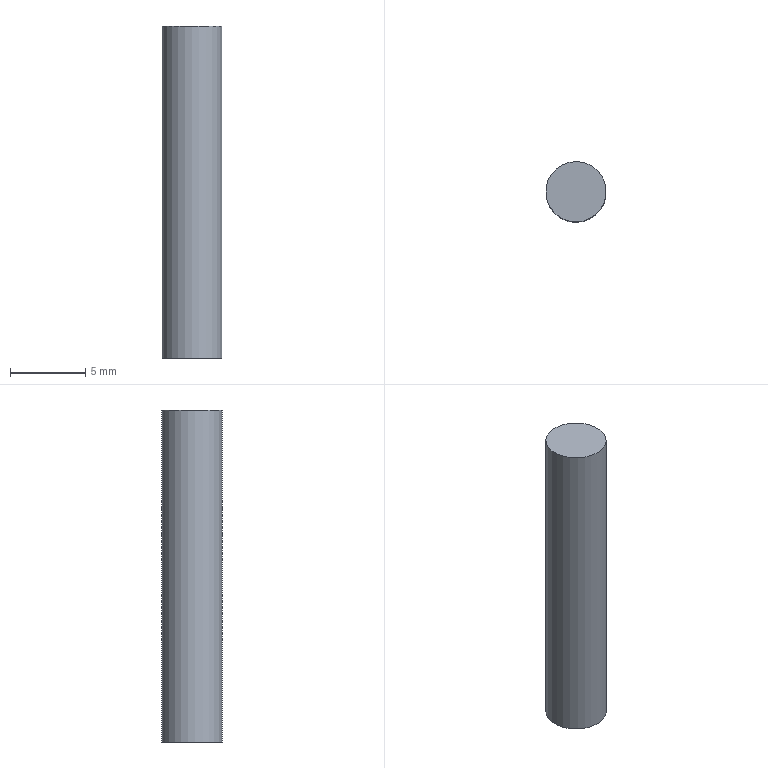Part | NX | features solid 2 | 1 solid | 3 faces | box 4 x 4 x 22 mm | volume 276.46 mm3 | plane 2 | cylinder 1 | commonest cylinder face diameters 4 x1
STEP:
#1=CARTESIAN_POINT('',(-819.874,-95.045,29.));
#2=VERTEX_POINT('',#1);
#3=CARTESIAN_POINT('',(-818.236,-96.192,29.));
#4=DIRECTION('',(0.,0.,1.));
#5=DIRECTION('',(-0.8192,0.5736,0.));
#6=AXIS2_PLACEMENT_3D('',#3,#4,#5);
#7=CIRCLE('',#6,2.);
#8=EDGE_CURVE('',#2,#2,#7,.T.);
#9=ORIENTED_EDGE('',*,*,#8,.F.);
#10=EDGE_LOOP('',(#9));
#11=FACE_BOUND('',#10,.T.);
#12=CARTESIAN_POINT('',(-818.236,-96.192,29.));
#13=DIRECTION('',(0.,0.,-1.));
#14=DIRECTION('',(0.8192,-0.5736,0.));
#15=AXIS2_PLACEMENT_3D('',#12,#13,#14);
#16=PLANE('',#15);
#17=ADVANCED_FACE('',(#11),#16,.T.);
#18=CARTESIAN_POINT('',(-816.597,-97.339,51.));
#19=VERTEX_POINT('',#18);
#20=CARTESIAN_POINT('',(-818.236,-96.192,51.));
#21=DIRECTION('',(0.,0.,-1.));
#22=DIRECTION('',(0.8192,-0.5736,0.));
#23=AXIS2_PLACEMENT_3D('',#20,#21,#22);
#24=CIRCLE('',#23,2.);
#25=EDGE_CURVE('',#19,#19,#24,.T.);
#26=ORIENTED_EDGE('',*,*,#25,.F.);
#27=EDGE_LOOP('',(#26));
#28=FACE_BOUND('',#27,.T.);
#29=CARTESIAN_POINT('',(-818.236,-96.192,51.));
#30=DIRECTION('',(0.,0.,1.));
#31=DIRECTION('',(-0.8192,0.5736,0.));
#32=AXIS2_PLACEMENT_3D('',#29,#30,#31);
#33=PLANE('',#32);
#34=ADVANCED_FACE('',(#28),#33,.T.);
#35=ORIENTED_EDGE('',*,*,#8,.T.);
#36=EDGE_LOOP('',(#35));
#37=FACE_BOUND('',#36,.T.);
#38=ORIENTED_EDGE('',*,*,#25,.T.);
#39=EDGE_LOOP('',(#38));
#40=FACE_BOUND('',#39,.T.);
#41=CARTESIAN_POINT('',(-818.236,-96.192,51.));
#42=DIRECTION('',(0.,0.,-1.));
#43=DIRECTION('',(0.8192,-0.5736,0.));
#44=AXIS2_PLACEMENT_3D('',#41,#42,#43);
#45=CYLINDRICAL_SURFACE('',#44,2.);
#46=ADVANCED_FACE('',(#37,#40),#45,.T.);
#47=CLOSED_SHELL('',(#17,#34,#46));
#48=MANIFOLD_SOLID_BREP('',#47);
#49=(LENGTH_UNIT()NAMED_UNIT(*)SI_UNIT(.MILLI.,.METRE.));
#50=UNCERTAINTY_MEASURE_WITH_UNIT(LENGTH_MEASURE(0.00001),#49,'','');
#51=(NAMED_UNIT(*)PLANE_ANGLE_UNIT()SI_UNIT($,.RADIAN.));
#52=(NAMED_UNIT(*)SI_UNIT($,.STERADIAN.)SOLID_ANGLE_UNIT());
#53=(GEOMETRIC_REPRESENTATION_CONTEXT(3)GLOBAL_UNCERTAINTY_ASSIGNED_CONTEXT((#50))GLOBAL_UNIT_ASSIGNED_CONTEXT((#49,#51,#52))REPRESENTATION_CONTEXT('',''));
#54=ADVANCED_BREP_SHAPE_REPRESENTATION('',(#48),#53);